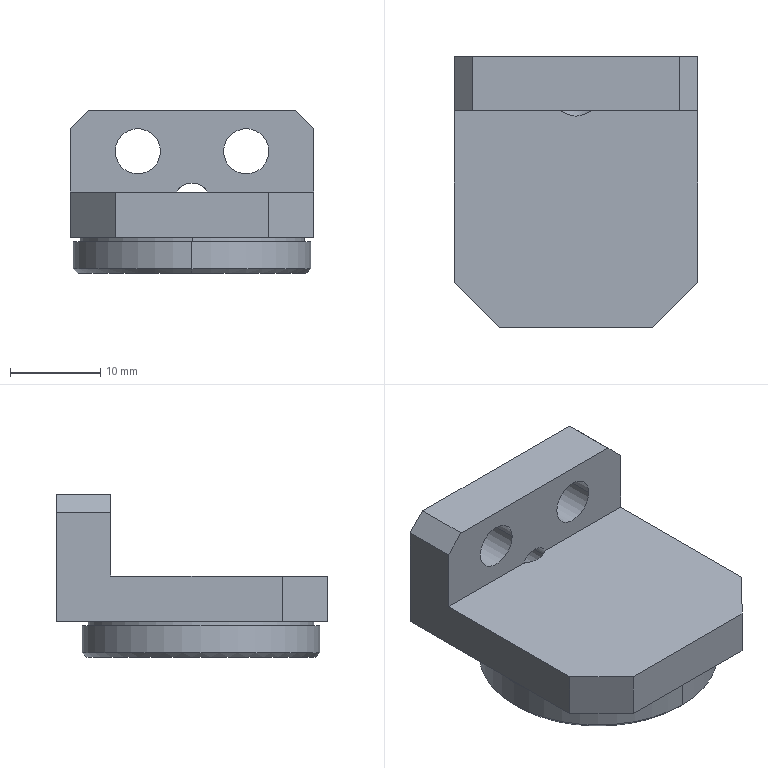NC program | NX | posted with a generic post | part box 27 x 30 x 18 mm
Whole program:
N10 G17 G21 G94 G90
(FLOOR_WALL_COPY , TOOL : D10JING)
N12 T11 M6
N14 G54
N16 G17 G0 G90 X23. Y-13.497 B0. C0. S9500 M3
N18 G43 Z30. H11
N20 Z9.5
N22 G94 G1 Z6.5 F1250.
N24 X20.
N26 X-20.
N28 Y-11.587
N30 Y-8.898
N32 X20.
N34 Y-4.298
N36 X-20.
N38 Y0.301
N40 X20.
N42 Y4.901
N44 X-20.
N46 Y9.5
N48 X20.
N50 X23.
N52 Z9.5
N54 G0 Z30.
N56 Y-13.497
N58 Z9.
N60 G1 Z6.
N62 X20.
N64 X-20.
N66 Y-11.587
N68 Y-8.898
N70 X20.
N72 Y-4.298
N74 X-20.
N76 Y0.301
N78 X20.
N80 Y4.901
N82 X-20.
N84 Y9.5
N86 X20.
N88 X23.
N90 Z9.
N92 G0 Z30.
N94 Y-13.497
N96 Z8.5
N98 G1 Z5.5
N100 X20.
N102 X-20.
N104 Y-11.587
N106 Y-8.898
N108 X20.
N110 Y-4.298
N112 X-20.
N114 Y0.301
N116 X20.
N118 Y4.901
N120 X-20.
N122 Y9.5
N124 X20.
N126 X23.
N128 Z8.5
N130 G0 Z30.
N132 Y-13.497
N134 Z8.
N136 G1 Z5.
N138 X20.
N140 X-20.
N142 Y-11.587
N144 Y-8.898
N146 X20.
N148 Y-4.298
N150 X-20.
N152 Y0.301
N154 X20.
N156 Y4.901
N158 X-20.
N160 Y9.5
N162 X20.
N164 X23.
N166 Z8.
N168 G0 Z30.
N170 Y-13.497
N172 Z7.5
N174 G1 Z4.5
N176 X20.
N178 X-20.
N180 Y-8.898
N182 X20.
N184 Y-4.298
N186 X-20.
N188 Y0.301
N190 X20.
N192 Y4.901
N194 X-20.
N196 Y9.5
N198 X20.
N200 X23.
N202 Z7.5
N204 G0 Z30.
N206 Y-13.497
N208 Z7.
N210 G1 Z4.
N212 X20.
N214 X-20.
N216 Y-8.898
N218 X20.
N220 Y-4.298
N222 X-20.
N224 Y0.301
N226 X20.
N228 Y4.901
N230 X-20.
N232 Y9.5
N234 X20.
N236 X23.
N238 Z7.
N240 G0 Z30.
N242 Y-13.497
N244 Z6.5
N246 G1 Z3.5
N248 X20.
N250 X-20.
N252 Y-8.898
N254 X20.
N256 Y-4.298
N258 X-20.
N260 Y0.301
N262 X20.
N264 Y4.901
N266 X-20.
N268 Y9.5
N270 X20.
N272 X23.
N274 Z6.5
N276 G0 Z30.
N278 Y-13.497
N280 Z6.
N282 G1 Z3.
N284 X20.
N286 X-20.
N288 Y-8.898
N290 X20.
N292 Y-4.298
N294 X-20.
N296 Y0.301
N298 X20.
N300 Y4.901
N302 X-20.
N304 Y9.5
N306 X20.
N308 X23.
N310 Z6.
N312 G0 Z30.
N314 Y-13.497
N316 Z5.5
N318 G1 Z2.5
N320 X20.
N322 X-20.
N324 Y-8.898
N326 X20.
N328 Y-4.298
N330 X-20.
N332 Y0.301
N334 X20.
N336 Y4.901
N338 X-20.
N340 Y9.5
N342 X20.
N344 X23.
N346 Z5.5
N348 G0 Z30.
N350 Y-13.497
N352 Z5.
N354 G1 Z2.
N356 X20.
N358 X-20.
N360 Y-8.898
N362 X20.
N364 Y-4.298
N366 X-20.
N368 Y0.301
N370 X20.
N372 Y4.901
N374 X-20.
N376 Y9.5
N378 X20.
N380 X23.
N382 Z5.
N384 G0 Z30.
N386 Y-13.497
N388 Z4.5
N390 G1 Z1.5
N392 X20.
N394 X-20.
N396 Y-8.898
N398 X20.
N400 Y-4.298
N402 X-20.
N404 Y0.301
N406 X20.
N408 Y4.901
N410 X-20.
N412 Y9.5
N414 X20.
N416 X23.
N418 Z4.5
N420 G0 Z30.
N422 Y-13.497
N424 Z4.
N426 G1 Z1.
N428 X20.
N430 X-20.
N432 Y-8.898
N434 X20.
N436 Y-4.298
N438 X-20.
N440 Y0.301
N442 X20.
N444 Y4.901
N446 X-20.
N448 Y9.5
N450 X20.
N452 X23.
N454 Z4.
N456 G0 Z30.
N458 Y-13.497
N460 Z3.5
N462 G1 Z0.5
N464 X20.
N466 X-20.
N468 Y-8.898
N470 X20.
N472 Y-4.298
N474 X-20.
N476 Y0.301
N478 X20.
N480 Y4.901
N482 X-20.
N484 Y9.5
N486 X20.
N488 X23.
N490 Z3.5
N492 G0 Z30.
N494 Y-13.497
N496 Z3.
N498 G1 Z0.
N500 X20.
N502 X-20.
N504 Y-8.898
N506 X20.
N508 Y-4.298
N510 X-20.
N512 Y0.301
N514 X20.
N516 Y4.901
N518 X-20.
N520 Y9.5
N522 X20.
N524 X23.
N526 Z3.
N528 G0 Z30.
N530 M5
(ZLEVEL_PROFILE_COPY , TOOL : D10)
N532 T10 M6
N534 G54
N536 G17 G0 G90 X16.827 Y9.07 B0. C0. S9500 M3
N538 G43 Z30. H10
N540 Z1.5
N542 G94 G1 X17.37 Y8.078 Z1.441 F1000.
N544 X17.997 Y6.66 Z1.359
N546 X18.501 Y5.193 Z1.278
N548 X18.878 Y3.689 Z1.197
N550 X19.127 Y2.158 Z1.116
N552 X19.245 Y0.611 Z1.034
N554 Y-0.597 Z0.971
N556 X19.11 Y-2.297 Z0.882
N558 X18.817 Y-3.977 Z0.792
N560 X18.368 Y-5.622 Z0.703
N562 X17.767 Y-7.219 Z0.614
N564 X17.02 Y-8.752 Z0.524
N566 X16.134 Y-10.209 Z0.435
N568 X15.115 Y-11.576 Z0.345
N570 X13.973 Y-12.843 Z0.256
N572 X12.718 Y-13.998 Z0.167
N574 X11.361 Y-15.03 Z0.077
N576 X10.796 Y-15.392 Z0.042
N578 X10.229 Y-15.75 Z0.007
N580 X8.895 Y-16.46 Z-0.072
N582 X7.506 Y-17.056 Z-0.151
N584 X6.073 Y-17.536 Z-0.231
N586 X4.604 Y-17.896 Z-0.31
N588 X3.112 Y-18.132 Z-0.389
N590 X1.604 Y-18.245 Z-0.468
N592 X1. Z-0.5
N594 G2 X-17.245 Y0. R18.245 F3000.
N596 X1. Y-18.245 R-18.245
N598 G1 X0.776 Y-18.244 Z-0.504
N600 X0.552 Y-18.24 Z-0.508
N602 X0.329 Y-18.233 Z-0.512
N604 X0.105 Y-18.223 Z-0.516
N606 X-0.118 Y-18.211 Z-0.52
N608 X-0.342 Y-18.196 Z-0.523
N610 X-0.565 Y-18.178 Z-0.527
N612 X-0.787 Y-18.157 Z-0.531
N614 X-1.01 Y-18.134 Z-0.535
N616 X-1.232 Y-18.108 Z-0.539
N618 X-1.454 Y-18.079 Z-0.543
N620 X-1.676 Y-18.048 Z-0.547
N622 X-1.897 Y-18.014 Z-0.551
N624 X-2.118 Y-17.977 Z-0.555
N626 X-2.338 Y-17.937 Z-0.559
N628 X-2.558 Y-17.895 Z-0.563
N630 X-2.777 Y-17.85 Z-0.566
N632 X-2.996 Y-17.802 Z-0.57
N634 X-3.214 Y-17.752 Z-0.574
N636 X-3.431 Y-17.699 Z-0.578
N638 X-3.648 Y-17.643 Z-0.582
N640 X-3.864 Y-17.585 Z-0.586
N642 X-4.079 Y-17.524 Z-0.59
N644 X-4.294 Y-17.46 Z-0.594
N646 X-4.507 Y-17.394 Z-0.598
N648 X-4.72 Y-17.325 Z-0.602
N650 X-4.932 Y-17.254 Z-0.605
N652 X-5.144 Y-17.18 Z-0.609
N654 X-5.354 Y-17.103 Z-0.613
N656 X-5.563 Y-17.024 Z-0.617
N658 X-5.772 Y-16.942 Z-0.621
N660 X-5.979 Y-16.858 Z-0.625
N662 X-6.185 Y-16.771 Z-0.629
N664 X-6.39 Y-16.681 Z-0.633
N666 X-6.594 Y-16.589 Z-0.637
N668 X-6.797 Y-16.495 Z-0.641
N670 X-6.999 Y-16.398 Z-0.645
N672 X-7.199 Y-16.299 Z-0.648
N674 X-7.399 Y-16.197 Z-0.652
N676 X-7.597 Y-16.093 Z-0.656
N678 X-7.793 Y-15.986 Z-0.66
N680 X-7.989 Y-15.877 Z-0.664
N682 X-8.183 Y-15.766 Z-0.668
N684 X-8.376 Y-15.652 Z-0.672
N686 X-8.567 Y-15.536 Z-0.676
N688 X-8.757 Y-15.417 Z-0.68
N690 X-8.945 Y-15.296 Z-0.684
N692 X-9.132 Y-15.173 Z-0.688
N694 X-9.317 Y-15.048 Z-0.691
N696 X-9.501 Y-14.92 Z-0.695
N698 X-9.683 Y-14.79 Z-0.699
N700 X-9.864 Y-14.658 Z-0.703
N702 X-10.043 Y-14.524 Z-0.707
N704 X-10.22 Y-14.387 Z-0.711
N706 X-10.396 Y-14.248 Z-0.715
N708 X-10.57 Y-14.108 Z-0.719
N710 X-10.742 Y-13.965 Z-0.723
N712 X-10.912 Y-13.819 Z-0.727
N714 X-11.081 Y-13.672 Z-0.73
N716 X-11.248 Y-13.523 Z-0.734
N718 X-11.413 Y-13.372 Z-0.738
N720 X-11.576 Y-13.219 Z-0.742
N722 X-11.737 Y-13.063 Z-0.746
N724 X-11.896 Y-12.906 Z-0.75
N726 X-12.053 Y-12.747 Z-0.754
N728 X-12.209 Y-12.586 Z-0.758
N730 X-12.362 Y-12.423 Z-0.762
N732 X-12.514 Y-12.258 Z-0.766
N734 X-12.663 Y-12.092 Z-0.77
N736 X-12.81 Y-11.923 Z-0.773
N738 X-12.955 Y-11.753 Z-0.777
N740 X-13.099 Y-11.581 Z-0.781
N742 X-13.239 Y-11.407 Z-0.785
N744 X-13.378 Y-11.231 Z-0.789
N746 X-13.515 Y-11.054 Z-0.793
N748 X-13.649 Y-10.875 Z-0.797
N750 X-13.782 Y-10.695 Z-0.801
N752 X-13.912 Y-10.513 Z-0.805
N754 X-14.04 Y-10.329 Z-0.809
N756 X-14.165 Y-10.144 Z-0.813
N758 X-14.289 Y-9.957 Z-0.816
N760 X-14.41 Y-9.769 Z-0.82
N762 X-14.528 Y-9.579 Z-0.824
N764 X-14.644 Y-9.388 Z-0.828
N766 X-14.758 Y-9.195 Z-0.832
N768 X-14.87 Y-9.001 Z-0.836
N770 X-14.979 Y-8.806 Z-0.84
N772 X-15.086 Y-8.609 Z-0.844
N774 X-15.19 Y-8.411 Z-0.848
N776 X-15.292 Y-8.212 Z-0.852
N778 X-15.392 Y-8.012 Z-0.855
N780 X-15.489 Y-7.81 Z-0.859
N782 X-15.583 Y-7.607 Z-0.863
N784 X-15.676 Y-7.403 Z-0.867
N786 X-15.765 Y-7.198 Z-0.871
N788 X-15.852 Y-6.992 Z-0.875
N790 X-15.937 Y-6.785 Z-0.879
N792 X-16.019 Y-6.576 Z-0.883
N794 X-16.098 Y-6.367 Z-0.887
N796 X-16.175 Y-6.157 Z-0.891
N798 X-16.249 Y-5.946 Z-0.895
N800 X-16.321 Y-5.734 Z-0.898
N802 X-16.39 Y-5.521 Z-0.902
N804 X-16.456 Y-5.307 Z-0.906
N806 X-16.52 Y-5.093 Z-0.91
N808 X-16.581 Y-4.878 Z-0.914
N810 X-16.639 Y-4.662 Z-0.918
N812 X-16.695 Y-4.445 Z-0.922
N814 X-16.748 Y-4.227 Z-0.926
N816 X-16.799 Y-4.009 Z-0.93
N818 X-16.847 Y-3.791 Z-0.934
N820 X-16.892 Y-3.572 Z-0.938
N822 X-16.934 Y-3.352 Z-0.941
N824 X-16.974 Y-3.132 Z-0.945
N826 X-17.011 Y-2.911 Z-0.949
N828 X-17.046 Y-2.69 Z-0.953
N830 X-17.077 Y-2.468 Z-0.957
N832 X-17.106 Y-2.246 Z-0.961
N834 X-17.132 Y-2.024 Z-0.965
N836 X-17.156 Y-1.802 Z-0.969
N838 X-17.177 Y-1.579 Z-0.973
N840 X-17.195 Y-1.356 Z-0.977
N842 X-17.21 Y-1.132 Z-0.98
N844 X-17.222 Y-0.909 Z-0.984
N846 X-17.232 Y-0.685 Z-0.988
N848 X-17.239 Y-0.462 Z-0.992
N850 X-17.243 Y-0.238 Z-0.996
N852 X-17.245 Y-0.014 Z-1.
N854 Y0.007
N856 G2 X1. Y-18.245 R-18.245
N858 G1 X0.776 Y-18.244 Z-1.004
N860 X0.552 Y-18.24 Z-1.008
N862 X0.329 Y-18.233 Z-1.012
N864 X0.105 Y-18.223 Z-1.016
N866 X-0.118 Y-18.211 Z-1.02
N868 X-0.342 Y-18.196 Z-1.023
N870 X-0.565 Y-18.178 Z-1.027
N872 X-0.787 Y-18.157 Z-1.031
N874 X-1.01 Y-18.134 Z-1.035
N876 X-1.232 Y-18.108 Z-1.039
N878 X-1.454 Y-18.079 Z-1.043
N880 X-1.676 Y-18.048 Z-1.047
N882 X-1.897 Y-18.014 Z-1.051
N884 X-2.118 Y-17.977 Z-1.055
N886 X-2.338 Y-17.937 Z-1.059
N888 X-2.558 Y-17.895 Z-1.063
N890 X-2.777 Y-17.85 Z-1.066
N892 X-2.996 Y-17.802 Z-1.07
N894 X-3.214 Y-17.752 Z-1.074
N896 X-3.431 Y-17.699 Z-1.078
N898 X-3.648 Y-17.643 Z-1.082
N900 X-3.864 Y-17.585 Z-1.086
N902 X-4.079 Y-17.524 Z-1.09
N904 X-4.294 Y-17.46 Z-1.094
N906 X-4.507 Y-17.394 Z-1.098
N908 X-4.72 Y-17.325 Z-1.102
N910 X-4.932 Y-17.254 Z-1.105
N912 X-5.144 Y-17.18 Z-1.109
N914 X-5.354 Y-17.103 Z-1.113
N916 X-5.563 Y-17.024 Z-1.117
N918 X-5.772 Y-16.942 Z-1.121
N920 X-5.979 Y-16.858 Z-1.125
N922 X-6.185 Y-16.771 Z-1.129
N924 X-6.39 Y-16.681 Z-1.133
N926 X-6.594 Y-16.589 Z-1.137
N928 X-6.797 Y-16.495 Z-1.141
N930 X-6.999 Y-16.398 Z-1.145
N932 X-7.199 Y-16.299 Z-1.148
N934 X-7.399 Y-16.197 Z-1.152
N936 X-7.597 Y-16.093 Z-1.156
N938 X-7.793 Y-15.986 Z-1.16
N940 X-7.989 Y-15.877 Z-1.164
N942 X-8.183 Y-15.766 Z-1.168
N944 X-8.376 Y-15.652 Z-1.172
N946 X-8.567 Y-15.536 Z-1.176
N948 X-8.757 Y-15.417 Z-1.18
N950 X-8.945 Y-15.296 Z-1.184
N952 X-9.132 Y-15.173 Z-1.188
N954 X-9.317 Y-15.048 Z-1.191
N956 X-9.501 Y-14.92 Z-1.195
N958 X-9.683 Y-14.79 Z-1.199
N960 X-9.864 Y-14.658 Z-1.203
N962 X-10.043 Y-14.524 Z-1.207
N964 X-10.22 Y-14.387 Z-1.211
N966 X-10.396 Y-14.248 Z-1.215
N968 X-10.57 Y-14.108 Z-1.219
N970 X-10.742 Y-13.965 Z-1.223
N972 X-10.912 Y-13.819 Z-1.227
N974 X-11.081 Y-13.672 Z-1.23
N976 X-11.248 Y-13.523 Z-1.234
N978 X-11.413 Y-13.372 Z-1.238
N980 X-11.576 Y-13.219 Z-1.242
N982 X-11.737 Y-13.063 Z-1.246
N984 X-11.896 Y-12.906 Z-1.25
N986 X-12.053 Y-12.747 Z-1.254
N988 X-12.209 Y-12.586 Z-1.258
N990 X-12.362 Y-12.423 Z-1.262
N992 X-12.514 Y-12.258 Z-1.266
N994 X-12.663 Y-12.092 Z-1.27
N996 X-12.81 Y-11.923 Z-1.273
N998 X-12.955 Y-11.753 Z-1.277
N1000 X-13.099 Y-11.581 Z-1.281
N1002 X-13.239 Y-11.407 Z-1.285
N1004 X-13.378 Y-11.231 Z-1.289
N1006 X-13.515 Y-11.054 Z-1.293
N1008 X-13.649 Y-10.875 Z-1.297
N1010 X-13.782 Y-10.695 Z-1.301
N1012 X-13.912 Y-10.513 Z-1.305
N1014 X-14.04 Y-10.329 Z-1.309
N1016 X-14.165 Y-10.144 Z-1.313
N1018 X-14.289 Y-9.957 Z-1.316
N1020 X-14.41 Y-9.769 Z-1.32
N1022 X-14.528 Y-9.579 Z-1.324
N1024 X-14.644 Y-9.388 Z-1.328
N1026 X-14.758 Y-9.195 Z-1.332
N1028 X-14.87 Y-9.001 Z-1.336
N1030 X-14.979 Y-8.806 Z-1.34
N1032 X-15.086 Y-8.609 Z-1.344
N1034 X-15.19 Y-8.411 Z-1.348
N1036 X-15.292 Y-8.212 Z-1.352
N1038 X-15.392 Y-8.012 Z-1.355
N1040 X-15.489 Y-7.81 Z-1.359
N1042 X-15.583 Y-7.607 Z-1.363
N1044 X-15.676 Y-7.403 Z-1.367
N1046 X-15.765 Y-7.198 Z-1.371
N1048 X-15.852 Y-6.992 Z-1.375
N1050 X-15.937 Y-6.785 Z-1.379
N1052 X-16.019 Y-6.576 Z-1.383
N1054 X-16.098 Y-6.367 Z-1.387
N1056 X-16.175 Y-6.157 Z-1.391
N1058 X-16.249 Y-5.946 Z-1.395
N1060 X-16.321 Y-5.734 Z-1.398
N1062 X-16.39 Y-5.521 Z-1.402
N1064 X-16.456 Y-5.307 Z-1.406
N1066 X-16.52 Y-5.093 Z-1.41
N1068 X-16.581 Y-4.878 Z-1.414
N1070 X-16.639 Y-4.662 Z-1.418
N1072 X-16.695 Y-4.445 Z-1.422
N1074 X-16.748 Y-4.227 Z-1.426
N1076 X-16.799 Y-4.009 Z-1.43
N1078 X-16.847 Y-3.791 Z-1.434
N1080 X-16.892 Y-3.572 Z-1.438
N1082 X-16.934 Y-3.352 Z-1.441
N1084 X-16.974 Y-3.132 Z-1.445
N1086 X-17.011 Y-2.911 Z-1.449
N1088 X-17.046 Y-2.69 Z-1.453
N1090 X-17.077 Y-2.468 Z-1.457
N1092 X-17.106 Y-2.246 Z-1.461
N1094 X-17.132 Y-2.024 Z-1.465
N1096 X-17.156 Y-1.802 Z-1.469
N1098 X-17.177 Y-1.579 Z-1.473
N1100 X-17.195 Y-1.356 Z-1.477
N1102 X-17.21 Y-1.132 Z-1.48
N1104 X-17.222 Y-0.909 Z-1.484
N1106 X-17.232 Y-0.685 Z-1.488
N1108 X-17.239 Y-0.462 Z-1.492
N1110 X-17.243 Y-0.238 Z-1.496
N1112 X-17.245 Y-0.014 Z-1.5
N1114 Y0.007
N1116 G2 X1. Y-18.245 R-18.245
N1118 G1 X0.776 Y-18.244 Z-1.504
N1120 X0.552 Y-18.24 Z-1.508
N1122 X0.329 Y-18.233 Z-1.512
N1124 X0.105 Y-18.223 Z-1.516
N1126 X-0.118 Y-18.211 Z-1.52
N1128 X-0.342 Y-18.196 Z-1.523
N1130 X-0.565 Y-18.178 Z-1.527
N1132 X-0.787 Y-18.157 Z-1.531
N1134 X-1.01 Y-18.134 Z-1.535
N1136 X-1.232 Y-18.108 Z-1.539
N1138 X-1.454 Y-18.079 Z-1.543
N1140 X-1.676 Y-18.048 Z-1.547
N1142 X-1.897 Y-18.014 Z-1.551
N1144 X-2.118 Y-17.977 Z-1.555
N1146 X-2.338 Y-17.937 Z-1.559
N1148 X-2.558 Y-17.895 Z-1.563
N1150 X-2.777 Y-17.85 Z-1.566
N1152 X-2.996 Y-17.802 Z-1.57
N1154 X-3.214 Y-17.752 Z-1.574
N1156 X-3.431 Y-17.699 Z-1.578
N1158 X-3.648 Y-17.643 Z-1.582
N1160 X-3.864 Y-17.585 Z-1.586
N1162 X-4.079 Y-17.524 Z-1.59
N1164 X-4.294 Y-17.46 Z-1.594
N1166 X-4.507 Y-17.394 Z-1.598
N1168 X-4.72 Y-17.325 Z-1.602
N1170 X-4.932 Y-17.254 Z-1.605
N1172 X-5.144 Y-17.18 Z-1.609
N1174 X-5.354 Y-17.103 Z-1.613
N1176 X-5.563 Y-17.024 Z-1.617
N1178 X-5.772 Y-16.942 Z-1.621
N1180 X-5.979 Y-16.858 Z-1.625
N1182 X-6.185 Y-16.771 Z-1.629
N1184 X-6.39 Y-16.681 Z-1.633
N1186 X-6.594 Y-16.589 Z-1.637
N1188 X-6.797 Y-16.495 Z-1.641
N1190 X-6.999 Y-16.398 Z-1.645
N1192 X-7.199 Y-16.299 Z-1.648
N1194 X-7.399 Y-16.197 Z-1.652
N1196 X-7.597 Y-16.093 Z-1.656
N1198 X-7.793 Y-15.986 Z-1.66
N1200 X-7.989 Y-15.877 Z-1.664
N1202 X-8.183 Y-15.766 Z-1.668
N1204 X-8.376 Y-15.652 Z-1.672
N1206 X-8.567 Y-15.536 Z-1.676
N1208 X-8.757 Y-15.417 Z-1.68
N1210 X-8.945 Y-15.296 Z-1.684
N1212 X-9.132 Y-15.173 Z-1.688
N1214 X-9.317 Y-15.048 Z-1.691
N1216 X-9.501 Y-14.92 Z-1.695
N1218 X-9.683 Y-14.79 Z-1.699
N1220 X-9.864 Y-14.658 Z-1.703
N1222 X-10.043 Y-14.524 Z-1.707
N1224 X-10.22 Y-14.387 Z-1.711
N1226 X-10.396 Y-14.248 Z-1.715
N1228 X-10.57 Y-14.108 Z-1.719
N1230 X-10.742 Y-13.965 Z-1.723
N1232 X-10.912 Y-13.819 Z-1.727
N1234 X-11.081 Y-13.672 Z-1.73
N1236 X-11.248 Y-13.523 Z-1.734
N1238 X-11.413 Y-13.372 Z-1.738
N1240 X-11.576 Y-13.219 Z-1.742
N1242 X-11.737 Y-13.063 Z-1.746
N1244 X-11.896 Y-12.906 Z-1.75
N1246 X-12.053 Y-12.747 Z-1.754
N1248 X-12.209 Y-12.586 Z-1.758
N1250 X-12.362 Y-12.423 Z-1.762
N1252 X-12.514 Y-12.258 Z-1.766
N1254 X-12.663 Y-12.092 Z-1.77
N1256 X-12.81 Y-11.923 Z-1.773
N1258 X-12.955 Y-11.753 Z-1.777
N1260 X-13.099 Y-11.581 Z-1.781
N1262 X-13.239 Y-11.407 Z-1.785
N1264 X-13.378 Y-11.231 Z-1.789
N1266 X-13.515 Y-11.054 Z-1.793
N1268 X-13.649 Y-10.875 Z-1.797
N1270 X-13.782 Y-10.695 Z-1.801
N1272 X-13.912 Y-10.513 Z-1.805
N1274 X-14.04 Y-10.329 Z-1.809
N1276 X-14.165 Y-10.144 Z-1.813
N1278 X-14.289 Y-9.957 Z-1.816
N1280 X-14.41 Y-9.769 Z-1.82
N1282 X-14.528 Y-9.579 Z-1.824
N1284 X-14.644 Y-9.388 Z-1.828
N1286 X-14.758 Y-9.195 Z-1.832
N1288 X-14.87 Y-9.001 Z-1.836
N1290 X-14.979 Y-8.806 Z-1.84
N1292 X-15.086 Y-8.609 Z-1.844
N1294 X-15.19 Y-8.411 Z-1.848
N1296 X-15.292 Y-8.212 Z-1.852
N1298 X-15.392 Y-8.012 Z-1.855
N1300 X-15.489 Y-7.81 Z-1.859
N1302 X-15.583 Y-7.607 Z-1.863
N1304 X-15.676 Y-7.403 Z-1.867
N1306 X-15.765 Y-7.198 Z-1.871
N1308 X-15.852 Y-6.992 Z-1.875
N1310 X-15.937 Y-6.785 Z-1.879
N1312 X-16.019 Y-6.576 Z-1.883
N1314 X-16.098 Y-6.367 Z-1.887
N1316 X-16.175 Y-6.157 Z-1.891
N1318 X-16.249 Y-5.946 Z-1.895
N1320 X-16.321 Y-5.734 Z-1.898
N1322 X-16.39 Y-5.521 Z-1.902
N1324 X-16.456 Y-5.307 Z-1.906
N1326 X-16.52 Y-5.093 Z-1.91
N1328 X-16.581 Y-4.878 Z-1.914
N1330 X-16.639 Y-4.662 Z-1.918
N1332 X-16.695 Y-4.445 Z-1.922
N1334 X-16.748 Y-4.227 Z-1.926
N1336 X-16.799 Y-4.009 Z-1.93
N1338 X-16.847 Y-3.791 Z-1.934
N1340 X-16.892 Y-3.572 Z-1.938
N1342 X-16.934 Y-3.352 Z-1.941
N1344 X-16.974 Y-3.132 Z-1.945
N1346 X-17.011 Y-2.911 Z-1.949
N1348 X-17.046 Y-2.69 Z-1.953
N1350 X-17.077 Y-2.468 Z-1.957
N1352 X-17.106 Y-2.246 Z-1.961
N1354 X-17.132 Y-2.024 Z-1.965
N1356 X-17.156 Y-1.802 Z-1.969
N1358 X-17.177 Y-1.579 Z-1.973
N1360 X-17.195 Y-1.356 Z-1.977
N1362 X-17.21 Y-1.132 Z-1.98
N1364 X-17.222 Y-0.909 Z-1.984
N1366 X-17.232 Y-0.685 Z-1.988
N1368 X-17.239 Y-0.462 Z-1.992
N1370 X-17.243 Y-0.238 Z-1.996
N1372 X-17.245 Y-0.014 Z-2.
N1374 Y0.007
N1376 G2 X1. Y-18.245 R-18.245
N1378 G1 X0.776 Y-18.244 Z-2.004
N1380 X0.552 Y-18.24 Z-2.008
N1382 X0.329 Y-18.233 Z-2.012
N1384 X0.105 Y-18.223 Z-2.016
N1386 X-0.118 Y-18.211 Z-2.02
N1388 X-0.342 Y-18.196 Z-2.023
N1390 X-0.565 Y-18.178 Z-2.027
N1392 X-0.787 Y-18.157 Z-2.031
N1394 X-1.01 Y-18.134 Z-2.035
N1396 X-1.232 Y-18.108 Z-2.039
N1398 X-1.454 Y-18.079 Z-2.043
N1400 X-1.676 Y-18.048 Z-2.047
N1402 X-1.897 Y-18.014 Z-2.051
N1404 X-2.118 Y-17.977 Z-2.055
N1406 X-2.338 Y-17.937 Z-2.059
N1408 X-2.558 Y-17.895 Z-2.063
N1410 X-2.777 Y-17.85 Z-2.066
N1412 X-2.996 Y-17.802 Z-2.07
N1414 X-3.214 Y-17.752 Z-2.074
N1416 X-3.431 Y-17.699 Z-2.078
N1418 X-3.648 Y-17.643 Z-2.082
N1420 X-3.864 Y-17.585 Z-2.086
N1422 X-4.079 Y-17.524 Z-2.09
N1424 X-4.294 Y-17.46 Z-2.094
N1426 X-4.507 Y-17.394 Z-2.098
N1428 X-4.72 Y-17.325 Z-2.102
N1430 X-4.932 Y-17.254 Z-2.105
N1432 X-5.144 Y-17.18 Z-2.109
N1434 X-5.354 Y-17.103 Z-2.113
N1436 X-5.563 Y-17.024 Z-2.117
N1438 X-5.772 Y-16.942 Z-2.121
N1440 X-5.979 Y-16.858 Z-2.125
N1442 X-6.185 Y-16.771 Z-2.129
N1444 X-6.39 Y-16.681 Z-2.133
N1446 X-6.594 Y-16.589 Z-2.137
N1448 X-6.797 Y-16.495 Z-2.141
N1450 X-6.999 Y-16.398 Z-2.145
N1452 X-7.199 Y-16.299 Z-2.148
N1454 X-7.399 Y-16.197 Z-2.152
N1456 X-7.597 Y-16.093 Z-2.156
N1458 X-7.793 Y-15.986 Z-2.16
N1460 X-7.989 Y-15.877 Z-2.164
N1462 X-8.183 Y-15.766 Z-2.168
N1464 X-8.376 Y-15.652 Z-2.172
N1466 X-8.567 Y-15.536 Z-2.176
N1468 X-8.757 Y-15.417 Z-2.18
N1470 X-8.945 Y-15.296 Z-2.184
N1472 X-9.132 Y-15.173 Z-2.188
N1474 X-9.317 Y-15.048 Z-2.191
N1476 X-9.501 Y-14.92 Z-2.195
N1478 X-9.683 Y-14.79 Z-2.199
N1480 X-9.864 Y-14.658 Z-2.203
N1482 X-10.043 Y-14.524 Z-2.207
N1484 X-10.22 Y-14.387 Z-2.211
N1486 X-10.396 Y-14.248 Z-2.215
N1488 X-10.57 Y-14.108 Z-2.219
N1490 X-10.742 Y-13.965 Z-2.223
N1492 X-10.912 Y-13.819 Z-2.227
N1494 X-11.081 Y-13.672 Z-2.23
N1496 X-11.248 Y-13.523 Z-2.234
N1498 X-11.413 Y-13.372 Z-2.238
N1500 X-11.576 Y-13.219 Z-2.242
N1502 X-11.737 Y-13.063 Z-2.246
N1504 X-11.896 Y-12.906 Z-2.25
N1506 X-12.053 Y-12.747 Z-2.254
N1508 X-12.209 Y-12.586 Z-2.258
N1510 X-12.362 Y-12.423 Z-2.262
N1512 X-12.514 Y-12.258 Z-2.266
N1514 X-12.663 Y-12.092 Z-2.27
N1516 X-12.81 Y-11.923 Z-2.273
N1518 X-12.955 Y-11.753 Z-2.277
N1520 X-13.099 Y-11.581 Z-2.281
N1522 X-13.239 Y-11.407 Z-2.285
N1524 X-13.378 Y-11.231 Z-2.289
N1526 X-13.515 Y-11.054 Z-2.293
N1528 X-13.649 Y-10.875 Z-2.297
N1530 X-13.782 Y-10.695 Z-2.301
N1532 X-13.912 Y-10.513 Z-2.305
N1534 X-14.04 Y-10.329 Z-2.309
N1536 X-14.165 Y-10.144 Z-2.313
N1538 X-14.289 Y-9.957 Z-2.316
N1540 X-14.41 Y-9.769 Z-2.32
N1542 X-14.528 Y-9.579 Z-2.324
N1544 X-14.644 Y-9.388 Z-2.328
N1546 X-14.758 Y-9.195 Z-2.332
N1548 X-14.87 Y-9.001 Z-2.336
N1550 X-14.979 Y-8.806 Z-2.34
N1552 X-15.086 Y-8.609 Z-2.344
N1554 X-15.19 Y-8.411 Z-2.348
N1556 X-15.292 Y-8.212 Z-2.352
N1558 X-15.392 Y-8.012 Z-2.355
N1560 X-15.489 Y-7.81 Z-2.359
N1562 X-15.583 Y-7.607 Z-2.363
N1564 X-15.676 Y-7.403 Z-2.367
N1566 X-15.765 Y-7.198 Z-2.371
N1568 X-15.852 Y-6.992 Z-2.375
N1570 X-15.937 Y-6.785 Z-2.379
N1572 X-16.019 Y-6.576 Z-2.383
N1574 X-16.098 Y-6.367 Z-2.387
N1576 X-16.175 Y-6.157 Z-2.391
N1578 X-16.249 Y-5.946 Z-2.395
N1580 X-16.321 Y-5.734 Z-2.398
N1582 X-16.39 Y-5.521 Z-2.402
N1584 X-16.456 Y-5.307 Z-2.406
N1586 X-16.52 Y-5.093 Z-2.41
N1588 X-16.581 Y-4.878 Z-2.414
N1590 X-16.639 Y-4.662 Z-2.418
N1592 X-16.695 Y-4.445 Z-2.422
N1594 X-16.748 Y-4.227 Z-2.426
N1596 X-16.799 Y-4.009 Z-2.43
N1598 X-16.847 Y-3.791 Z-2.434
N1600 X-16.892 Y-3.572 Z-2.438
N1602 X-16.934 Y-3.352 Z-2.441
N1604 X-16.974 Y-3.132 Z-2.445
N1606 X-17.011 Y-2.911 Z-2.449
N1608 X-17.046 Y-2.69 Z-2.453
N1610 X-17.077 Y-2.468 Z-2.457
N1612 X-17.106 Y-2.246 Z-2.461
N1614 X-17.132 Y-2.024 Z-2.465
N1616 X-17.156 Y-1.802 Z-2.469
N1618 X-17.177 Y-1.579 Z-2.473
N1620 X-17.195 Y-1.356 Z-2.477
N1622 X-17.21 Y-1.132 Z-2.48
N1624 X-17.222 Y-0.909 Z-2.484
N1626 X-17.232 Y-0.685 Z-2.488
N1628 X-17.239 Y-0.462 Z-2.492
N1630 X-17.243 Y-0.238 Z-2.496
N1632 X-17.245 Y-0.014 Z-2.5
N1634 Y0.007
N1636 G2 X1. Y-18.245 R-18.245
N1638 G1 X0.776 Y-18.244 Z-2.504
N1640 X0.552 Y-18.24 Z-2.508
N1642 X0.329 Y-18.233 Z-2.512
N1644 X0.105 Y-18.223 Z-2.516
N1646 X-0.118 Y-18.211 Z-2.52
N1648 X-0.342 Y-18.196 Z-2.523
N1650 X-0.565 Y-18.178 Z-2.527
N1652 X-0.787 Y-18.157 Z-2.531
N1654 X-1.01 Y-18.134 Z-2.535
N1656 X-1.232 Y-18.108 Z-2.539
N1658 X-1.454 Y-18.079 Z-2.543
N1660 X-1.676 Y-18.048 Z-2.547
N1662 X-1.897 Y-18.014 Z-2.551
N1664 X-2.118 Y-17.977 Z-2.555
N1666 X-2.338 Y-17.937 Z-2.559
N1668 X-2.558 Y-17.895 Z-2.563
N1670 X-2.777 Y-17.85 Z-2.566
N1672 X-2.996 Y-17.802 Z-2.57
N1674 X-3.214 Y-17.752 Z-2.574
N1676 X-3.431 Y-17.699 Z-2.578
N1678 X-3.648 Y-17.643 Z-2.582
N1680 X-3.864 Y-17.585 Z-2.586
N1682 X-4.079 Y-17.524 Z-2.59
N1684 X-4.294 Y-17.46 Z-2.594
N1686 X-4.507 Y-17.394 Z-2.598
N1688 X-4.72 Y-17.325 Z-2.602
N1690 X-4.932 Y-17.254 Z-2.605
N1692 X-5.144 Y-17.18 Z-2.609
N1694 X-5.354 Y-17.103 Z-2.613
N1696 X-5.563 Y-17.024 Z-2.617
N1698 X-5.772 Y-16.942 Z-2.621
N1700 X-5.979 Y-16.858 Z-2.625
N1702 X-6.185 Y-16.771 Z-2.629
N1704 X-6.39 Y-16.681 Z-2.633
N1706 X-6.594 Y-16.589 Z-2.637
N1708 X-6.797 Y-16.495 Z-2.641
N1710 X-6.999 Y-16.398 Z-2.645
N1712 X-7.199 Y-16.299 Z-2.648
N1714 X-7.399 Y-16.197 Z-2.652
N1716 X-7.597 Y-16.093 Z-2.656
N1718 X-7.793 Y-15.986 Z-2.66
N1720 X-7.989 Y-15.877 Z-2.664
N1722 X-8.183 Y-15.766 Z-2.668
N1724 X-8.376 Y-15.652 Z-2.672
N1726 X-8.567 Y-15.536 Z-2.676
N1728 X-8.757 Y-15.417 Z-2.68
N1730 X-8.945 Y-15.296 Z-2.684
N1732 X-9.132 Y-15.173 Z-2.688
N1734 X-9.317 Y-15.048 Z-2.691
N1736 X-9.501 Y-14.92 Z-2.695
N1738 X-9.683 Y-14.79 Z-2.699
N1740 X-9.864 Y-14.658 Z-2.703
N1742 X-10.043 Y-14.524 Z-2.707
N1744 X-10.22 Y-14.387 Z-2.711
N1746 X-10.396 Y-14.248 Z-2.715
N1748 X-10.57 Y-14.108 Z-2.719
N1750 X-10.742 Y-13.965 Z-2.723
N1752 X-10.912 Y-13.819 Z-2.727
N1754 X-11.081 Y-13.672 Z-2.73
N1756 X-11.248 Y-13.523 Z-2.734
N1758 X-11.413 Y-13.372 Z-2.738
N1760 X-11.576 Y-13.219 Z-2.742
N1762 X-11.737 Y-13.063 Z-2.746
N1764 X-11.896 Y-12.906 Z-2.75
N1766 X-12.053 Y-12.747 Z-2.754
N1768 X-12.209 Y-12.586 Z-2.758
N1770 X-12.362 Y-12.423 Z-2.762
N1772 X-12.514 Y-12.258 Z-2.766
N1774 X-12.663 Y-12.092 Z-2.77
N1776 X-12.81 Y-11.923 Z-2.773
N1778 X-12.955 Y-11.753 Z-2.777
N1780 X-13.099 Y-11.581 Z-2.781
N1782 X-13.239 Y-11.407 Z-2.785
N1784 X-13.378 Y-11.231 Z-2.789
N1786 X-13.515 Y-11.054 Z-2.793
N1788 X-13.649 Y-10.875 Z-2.797
N1790 X-13.782 Y-10.695 Z-2.801
N1792 X-13.912 Y-10.513 Z-2.805
N1794 X-14.04 Y-10.329 Z-2.809
N1796 X-14.165 Y-10.144 Z-2.813
N1798 X-14.289 Y-9.957 Z-2.816
N1800 X-14.41 Y-9.769 Z-2.82
N1802 X-14.528 Y-9.579 Z-2.824
N1804 X-14.644 Y-9.388 Z-2.828
N1806 X-14.758 Y-9.195 Z-2.832
N1808 X-14.87 Y-9.001 Z-2.836
N1810 X-14.979 Y-8.806 Z-2.84
N1812 X-15.086 Y-8.609 Z-2.844
N1814 X-15.19 Y-8.411 Z-2.848
N1816 X-15.292 Y-8.212 Z-2.852
N1818 X-15.392 Y-8.012 Z-2.855
N1820 X-15.489 Y-7.81 Z-2.859
N1822 X-15.583 Y-7.607 Z-2.863
N1824 X-15.676 Y-7.403 Z-2.867
N1826 X-15.765 Y-7.198 Z-2.871
N1828 X-15.852 Y-6.992 Z-2.875
N1830 X-15.937 Y-6.785 Z-2.879
N1832 X-16.019 Y-6.576 Z-2.883
N1834 X-16.098 Y-6.367 Z-2.887
N1836 X-16.175 Y-6.157 Z-2.891
N1838 X-16.249 Y-5.946 Z-2.895
N1840 X-16.321 Y-5.734 Z-2.898
N1842 X-16.39 Y-5.521 Z-2.902
N1844 X-16.456 Y-5.307 Z-2.906
N1846 X-16.52 Y-5.093 Z-2.91
N1848 X-16.581 Y-4.878 Z-2.914
N1850 X-16.639 Y-4.662 Z-2.918
N1852 X-16.695 Y-4.445 Z-2.922
N1854 X-16.748 Y-4.227 Z-2.926
N1856 X-16.799 Y-4.009 Z-2.93
N1858 X-16.847 Y-3.791 Z-2.934
N1860 X-16.892 Y-3.572 Z-2.938
N1862 X-16.934 Y-3.352 Z-2.941
N1864 X-16.974 Y-3.132 Z-2.945
N1866 X-17.011 Y-2.911 Z-2.949
N1868 X-17.046 Y-2.69 Z-2.953
N1870 X-17.077 Y-2.468 Z-2.957
N1872 X-17.106 Y-2.246 Z-2.961
N1874 X-17.132 Y-2.024 Z-2.965
N1876 X-17.156 Y-1.802 Z-2.969
N1878 X-17.177 Y-1.579 Z-2.973
N1880 X-17.195 Y-1.356 Z-2.977
N1882 X-17.21 Y-1.132 Z-2.98
N1884 X-17.222 Y-0.909 Z-2.984
N1886 X-17.232 Y-0.685 Z-2.988
N1888 X-17.239 Y-0.462 Z-2.992
N1890 X-17.243 Y-0.238 Z-2.996
N1892 X-17.245 Y-0.014 Z-3.
N1894 Y0.007
N1896 G2 X1. Y-18.245 R-18.245
N1898 G1 X0.776 Y-18.244 Z-3.004
N1900 X0.552 Y-18.24 Z-3.008
N1902 X0.329 Y-18.233 Z-3.012
N1904 X0.105 Y-18.223 Z-3.016
N1906 X-0.118 Y-18.211 Z-3.02
N1908 X-0.342 Y-18.196 Z-3.023
N1910 X-0.565 Y-18.178 Z-3.027
N1912 X-0.787 Y-18.157 Z-3.031
N1914 X-1.01 Y-18.134 Z-3.035
N1916 X-1.232 Y-18.108 Z-3.039
N1918 X-1.454 Y-18.079 Z-3.043
N1920 X-1.676 Y-18.048 Z-3.047
N1922 X-1.897 Y-18.014 Z-3.051
N1924 X-2.118 Y-17.977 Z-3.055
N1926 X-2.338 Y-17.937 Z-3.059
N1928 X-2.558 Y-17.895 Z-3.063
N1930 X-2.777 Y-17.85 Z-3.066
N1932 X-2.996 Y-17.802 Z-3.07
N1934 X-3.214 Y-17.752 Z-3.074
N1936 X-3.431 Y-17.699 Z-3.078
N1938 X-3.648 Y-17.643 Z-3.082
N1940 X-3.864 Y-17.585 Z-3.086
N1942 X-4.079 Y-17.524 Z-3.09
N1944 X-4.294 Y-17.46 Z-3.094
N1946 X-4.507 Y-17.394 Z-3.098
N1948 X-4.72 Y-17.325 Z-3.102
N1950 X-4.932 Y-17.254 Z-3.105
N1952 X-5.144 Y-17.18 Z-3.109
N1954 X-5.354 Y-17.103 Z-3.113
N1956 X-5.563 Y-17.024 Z-3.117
N1958 X-5.772 Y-16.942 Z-3.121
N1960 X-5.979 Y-16.858 Z-3.125
N1962 X-6.185 Y-16.771 Z-3.129
N1964 X-6.39 Y-16.681 Z-3.133
N1966 X-6.594 Y-16.589 Z-3.137
N1968 X-6.797 Y-16.495 Z-3.141
N1970 X-6.999 Y-16.398 Z-3.145
N1972 X-7.199 Y-16.299 Z-3.148
N1974 X-7.399 Y-16.197 Z-3.152
N1976 X-7.597 Y-16.093 Z-3.156
N1978 X-7.793 Y-15.986 Z-3.16
N1980 X-7.989 Y-15.877 Z-3.164
N1982 X-8.183 Y-15.766 Z-3.168
N1984 X-8.376 Y-15.652 Z-3.172
N1986 X-8.567 Y-15.536 Z-3.176
N1988 X-8.757 Y-15.417 Z-3.18
N1990 X-8.945 Y-15.296 Z-3.184
N1992 X-9.132 Y-15.173 Z-3.188
N1994 X-9.317 Y-15.048 Z-3.191
N1996 X-9.501 Y-14.92 Z-3.195
N1998 X-9.683 Y-14.79 Z-3.199
N2000 X-9.864 Y-14.658 Z-3.203
N2002 X-10.043 Y-14.524 Z-3.207
N2004 X-10.22 Y-14.387 Z-3.211
N2006 X-10.396 Y-14.248 Z-3.215
N2008 X-10.57 Y-14.108 Z-3.219
N2010 X-10.742 Y-13.965 Z-3.223
N2012 X-10.912 Y-13.819 Z-3.227
N2014 X-11.081 Y-13.672 Z-3.23
N2016 X-11.248 Y-13.523 Z-3.234
N2018 X-11.413 Y-13.372 Z-3.238
N2020 X-11.576 Y-13.219 Z-3.242
N2022 X-11.737 Y-13.063 Z-3.246
N2024 X-11.896 Y-12.906 Z-3.25
N2026 X-12.053 Y-12.747 Z-3.254
N2028 X-12.209 Y-12.586 Z-3.258
N2030 X-12.362 Y-12.423 Z-3.262
N2032 X-12.514 Y-12.258 Z-3.266
N2034 X-12.663 Y-12.092 Z-3.27
N2036 X-12.81 Y-11.923 Z-3.273
N2038 X-12.955 Y-11.753 Z-3.277
N2040 X-13.099 Y-11.581 Z-3.281
N2042 X-13.239 Y-11.407 Z-3.285
N2044 X-13.378 Y-11.231 Z-3.289
N2046 X-13.515 Y-11.054 Z-3.293
N2048 X-13.649 Y-10.875 Z-3.297
N2050 X-13.782 Y-10.695 Z-3.301
N2052 X-13.912 Y-10.513 Z-3.305
N2054 X-14.04 Y-10.329 Z-3.309
N2056 X-14.165 Y-10.144 Z-3.313
N2058 X-14.289 Y-9.957 Z-3.316
N2060 X-14.41 Y-9.769 Z-3.32
N2062 X-14.528 Y-9.579 Z-3.324
N2064 X-14.644 Y-9.388 Z-3.328
N2066 X-14.758 Y-9.195 Z-3.332
N2068 X-14.87 Y-9.001 Z-3.336
N2070 X-14.979 Y-8.806 Z-3.34
N2072 X-15.086 Y-8.609 Z-3.344
N2074 X-15.19 Y-8.411 Z-3.348
N2076 X-15.292 Y-8.212 Z-3.352
N2078 X-15.392 Y-8.012 Z-3.355
N2080 X-15.489 Y-7.81 Z-3.359
N2082 X-15.583 Y-7.607 Z-3.363
N2084 X-15.676 Y-7.403 Z-3.367
N2086 X-15.765 Y-7.198 Z-3.371
N2088 X-15.852 Y-6.992 Z-3.375
N2090 X-15.937 Y-6.785 Z-3.379
N2092 X-16.019 Y-6.576 Z-3.383
N2094 X-16.098 Y-6.367 Z-3.387
N2096 X-16.175 Y-6.157 Z-3.391
N2098 X-16.249 Y-5.946 Z-3.395
N2100 X-16.321 Y-5.734 Z-3.398
N2102 X-16.39 Y-5.521 Z-3.402
N2104 X-16.456 Y-5.307 Z-3.406
N2106 X-16.52 Y-5.093 Z-3.41
N2108 X-16.581 Y-4.878 Z-3.414
N2110 X-16.639 Y-4.662 Z-3.418
N2112 X-16.695 Y-4.445 Z-3.422
N2114 X-16.748 Y-4.227 Z-3.426
N2116 X-16.799 Y-4.009 Z-3.43
N2118 X-16.847 Y-3.791 Z-3.434
N2120 X-16.892 Y-3.572 Z-3.438
N2122 X-16.934 Y-3.352 Z-3.441
N2124 X-16.974 Y-3.132 Z-3.445
N2126 X-17.011 Y-2.911 Z-3.449
N2128 X-17.046 Y-2.69 Z-3.453
N2130 X-17.077 Y-2.468 Z-3.457
N2132 X-17.106 Y-2.246 Z-3.461
N2134 X-17.132 Y-2.024 Z-3.465
N2136 X-17.156 Y-1.802 Z-3.469
N2138 X-17.177 Y-1.579 Z-3.473
N2140 X-17.195 Y-1.356 Z-3.477
N2142 X-17.21 Y-1.132 Z-3.48
N2144 X-17.222 Y-0.909 Z-3.484
N2146 X-17.232 Y-0.685 Z-3.488
N2148 X-17.239 Y-0.462 Z-3.492
N2150 X-17.243 Y-0.238 Z-3.496
N2152 X-17.245 Y-0.014 Z-3.5
N2154 Y0.007
N2156 G2 X1. Y-18.245 R-18.245
N2158 G1 X0.776 Y-18.244 Z-3.504
N2160 X0.552 Y-18.24 Z-3.508
N2162 X0.329 Y-18.233 Z-3.512
N2164 X0.105 Y-18.223 Z-3.516
N2166 X-0.118 Y-18.211 Z-3.52
N2168 X-0.342 Y-18.196 Z-3.523
N2170 X-0.565 Y-18.178 Z-3.527
N2172 X-0.787 Y-18.157 Z-3.531
N2174 X-1.01 Y-18.134 Z-3.535
N2176 X-1.232 Y-18.108 Z-3.539
N2178 X-1.454 Y-18.079 Z-3.543
N2180 X-1.676 Y-18.048 Z-3.547
N2182 X-1.897 Y-18.014 Z-3.551
N2184 X-2.118 Y-17.977 Z-3.555
N2186 X-2.338 Y-17.937 Z-3.559
N2188 X-2.558 Y-17.895 Z-3.563
N2190 X-2.777 Y-17.85 Z-3.566
N2192 X-2.996 Y-17.802 Z-3.57
N2194 X-3.214 Y-17.752 Z-3.574
N2196 X-3.431 Y-17.699 Z-3.578
N2198 X-3.648 Y-17.643 Z-3.582
N2200 X-3.864 Y-17.585 Z-3.586
N2202 X-4.079 Y-17.524 Z-3.59
N2204 X-4.294 Y-17.46 Z-3.594
N2206 X-4.507 Y-17.394 Z-3.598
N2208 X-4.72 Y-17.325 Z-3.602
N2210 X-4.932 Y-17.254 Z-3.605
N2212 X-5.144 Y-17.18 Z-3.609
N2214 X-5.354 Y-17.103 Z-3.613
N2216 X-5.563 Y-17.024 Z-3.617
N2218 X-5.772 Y-16.942 Z-3.621
N2220 X-5.979 Y-16.858 Z-3.625
N2222 X-6.185 Y-16.771 Z-3.629
N2224 X-6.39 Y-16.681 Z-3.633
N2226 X-6.594 Y-16.589 Z-3.637
N2228 X-6.797 Y-16.495 Z-3.641
N2230 X-6.999 Y-16.398 Z-3.645
N2232 X-7.199 Y-16.299 Z-3.648
N2234 X-7.399 Y-16.197 Z-3.652
N2236 X-7.597 Y-16.093 Z-3.656
N2238 X-7.793 Y-15.986 Z-3.66
N2240 X-7.989 Y-15.877 Z-3.664
N2242 X-8.183 Y-15.766 Z-3.668
N2244 X-8.376 Y-15.652 Z-3.672
N2246 X-8.567 Y-15.536 Z-3.676
N2248 X-8.757 Y-15.417 Z-3.68
N2250 X-8.945 Y-15.296 Z-3.684
N2252 X-9.132 Y-15.173 Z-3.688
N2254 X-9.317 Y-15.048 Z-3.691
N2256 X-9.501 Y-14.92 Z-3.695
N2258 X-9.683 Y-14.79 Z-3.699
N2260 X-9.864 Y-14.658 Z-3.703
N2262 X-10.043 Y-14.524 Z-3.707
N2264 X-10.22 Y-14.387 Z-3.711
N2266 X-10.396 Y-14.248 Z-3.715
N2268 X-10.57 Y-14.108 Z-3.719
N2270 X-10.742 Y-13.965 Z-3.723
N2272 X-10.912 Y-13.819 Z-3.727
N2274 X-11.081 Y-13.672 Z-3.73
N2276 X-11.248 Y-13.523 Z-3.734
N2278 X-11.413 Y-13.372 Z-3.738
N2280 X-11.576 Y-13.219 Z-3.742
N2282 X-11.737 Y-13.063 Z-3.746
N2284 X-11.896 Y-12.906 Z-3.75
N2286 X-12.053 Y-12.747 Z-3.754
N2288 X-12.209 Y-12.586 Z-3.758
N2290 X-12.362 Y-12.423 Z-3.762
N2292 X-12.514 Y-12.258 Z-3.766
N2294 X-12.663 Y-12.092 Z-3.77
N2296 X-12.81 Y-11.923 Z-3.773
N2298 X-12.955 Y-11.753 Z-3.777
N2300 X-13.099 Y-11.581 Z-3.781
N2302 X-13.239 Y-11.407 Z-3.785
N2304 X-13.378 Y-11.231 Z-3.789
N2306 X-13.515 Y-11.054 Z-3.793
N2308 X-13.649 Y-10.875 Z-3.797
N2310 X-13.782 Y-10.695 Z-3.801
N2312 X-13.912 Y-10.513 Z-3.805
N2314 X-14.04 Y-10.329 Z-3.809
N2316 X-14.165 Y-10.144 Z-3.813
N2318 X-14.289 Y-9.957 Z-3.816
N2320 X-14.41 Y-9.769 Z-3.82
N2322 X-14.528 Y-9.579 Z-3.824
N2324 X-14.644 Y-9.388 Z-3.828
N2326 X-14.758 Y-9.195 Z-3.832
N2328 X-14.87 Y-9.001 Z-3.836
N2330 X-14.979 Y-8.806 Z-3.84
N2332 X-15.086 Y-8.609 Z-3.844
N2334 X-15.19 Y-8.411 Z-3.848
N2336 X-15.292 Y-8.212 Z-3.852
N2338 X-15.392 Y-8.012 Z-3.855
N2340 X-15.489 Y-7.81 Z-3.859
N2342 X-15.583 Y-7.607 Z-3.863
N2344 X-15.676 Y-7.403 Z-3.867
N2346 X-15.765 Y-7.198 Z-3.871
N2348 X-15.852 Y-6.992 Z-3.875
N2350 X-15.937 Y-6.785 Z-3.879
N2352 X-16.019 Y-6.576 Z-3.883
N2354 X-16.098 Y-6.367 Z-3.887
N2356 X-16.175 Y-6.157 Z-3.891
N2358 X-16.249 Y-5.946 Z-3.895
N2360 X-16.321 Y-5.734 Z-3.898
N2362 X-16.39 Y-5.521 Z-3.902
N2364 X-16.456 Y-5.307 Z-3.906
N2366 X-16.52 Y-5.093 Z-3.91
N2368 X-16.581 Y-4.878 Z-3.914
N2370 X-16.639 Y-4.662 Z-3.918
N2372 X-16.695 Y-4.445 Z-3.922
N2374 X-16.748 Y-4.227 Z-3.926
N2376 X-16.799 Y-4.009 Z-3.93
N2378 X-16.847 Y-3.791 Z-3.934
N2380 X-16.892 Y-3.572 Z-3.938
N2382 X-16.934 Y-3.352 Z-3.941
N2384 X-16.974 Y-3.132 Z-3.945
N2386 X-17.011 Y-2.911 Z-3.949
N2388 X-17.046 Y-2.69 Z-3.953
N2390 X-17.077 Y-2.468 Z-3.957
N2392 X-17.106 Y-2.246 Z-3.961
N2394 X-17.132 Y-2.024 Z-3.965
N2396 X-17.156 Y-1.802 Z-3.969
N2398 X-17.177 Y-1.579 Z-3.973
N2400 X-17.195 Y-1.356 Z-3.977
N2402 X-17.21 Y-1.132 Z-3.98
N2404 X-17.222 Y-0.909 Z-3.984
N2406 X-17.232 Y-0.685 Z-3.988
N2408 X-17.239 Y-0.462 Z-3.992
N2410 X-17.243 Y-0.238 Z-3.996
N2412 X-17.245 Y-0.014 Z-4.
N2414 Y0.007
N2416 G2 X1.007 Y18.245 R18.245
N2418 X-17.245 Y-0.014 R-18.245
N2420 G1 Z-2.5
N2422 G0 Z30.
N2424 M5
(ZLEVEL_PROFILE_COPY_1_COPY , TOOL : D10JING)
N2426 T11 M6
N2428 G54
N2430 G17 G0 G90 X2.691 Y-20.074 B0. C0. S9500 M3
N2432 G43 Z30. H11
N2434 Z-2.5
N2436 G94 G1 Z-4. F1000.
N2438 X1.866 Y-18.645
N2440 G3 X1. Y-18.145 R1.
N2442 G2 X-17.145 Y0. R18.145 F1200.
N2444 X1. Y-18.145 R-18.145
N2446 G3 X0.134 Y-18.645 R1.
N2448 G1 X-0.691 Y-20.074
N2450 Z-2.5
N2452 G0 Z30.
N2454 M5
(PLANAR_MILL_COPY_COPY_1 , TOOL : D6A45)
N2456 T07 M6
N2458 G54
N2460 G17 G0 G90 X15.793 Y1.24 B0. C0. S9500 M3
N2462 G43 Z30. H7
N2464 Z0.5
N2466 G94 G1 Z-1. F1250.
N2468 X15.145 Y0.866
N2470 G3 X14.645 Y0. R1.
N2472 G2 X1. Y-13.645 R13.645
N2474 X14.645 Y0. R-13.645
N2476 G3 X15.145 Y-0.866 R1.
N2478 G1 X15.793 Y-1.24
N2480 Z0.5
N2482 G0 Z30.
N2484 M5
(PLANAR_MILL , TOOL : T8H0.5)
N2486 T08 M6
N2488 G54
N2490 G17 G0 G90 X21.27 Y5.859 B0. C0. S5000 M3
N2492 G43 Z30. H8
N2494 Z-1.
N2496 G94 G1 Z-4. F1000.
N2498 G3 X18.1 Y0. R7.
N2500 G2 X1. Y-17.1 R17.1
N2502 X18.1 Y0. R-17.1
N2504 G3 X21.27 Y-5.859 R7.
N2506 G1 X21.262 Y5.887
N2508 G3 X18.05 Y0. R7.
N2510 G2 X1. Y-17.05 R17.05
N2512 X18.05 Y0. R-17.05
N2514 G3 X21.218 Y-5.858 R7.
N2516 G1 X21.21 Y5.886
N2518 G3 X18. Y0. R7.
N2520 G2 X1. Y-17. R17.
N2522 X18. Y0. R-17.
N2524 G3 X21.167 Y-5.857 R7.
N2526 G1 X21.159 Y5.884
N2528 G3 X17.95 Y0. R7.
N2530 G2 X1. Y-16.95 R16.95
N2532 X17.95 Y0. R-16.95
N2534 G3 X21.115 Y-5.856 R7.
N2536 G1 X21.107 Y5.883
N2538 G3 X17.9 Y0. R7.
N2540 G2 X1. Y-16.9 R16.9
N2542 X17.9 Y0. R-16.9
N2544 G3 X21.063 Y-5.855 R7.
N2546 G1 X21.055 Y5.882
N2548 G3 X17.85 Y0. R7.
N2550 G2 X1. Y-16.85 R16.85
N2552 X17.85 Y0. R-16.85
N2554 G3 X21.011 Y-5.854 R7.
N2556 G1 X21.003 Y5.881
N2558 G3 X17.8 Y0. R7.
N2560 G2 X1. Y-16.8 R16.8
N2562 X17.8 Y0. R-16.8
N2564 G3 X20.96 Y-5.853 R7.
N2566 G1 X20.952 Y5.88
N2568 G3 X17.75 Y0. R7.
N2570 G2 X1. Y-16.75 R16.75
N2572 X17.75 Y0. R-16.75
N2574 G3 X20.908 Y-5.851 R7.
N2576 G1 X20.9 Y5.879
N2578 G3 X17.7 Y0. R7.
N2580 G2 X1. Y-16.7 R16.7
N2582 X17.7 Y0. R-16.7
N2584 G3 X20.856 Y-5.85 R7.
N2586 G1 X20.848 Y5.878
N2588 G3 X17.65 Y0. R7.
N2590 G2 X1. Y-16.65 R16.65
N2592 X17.65 Y0. R-16.65
N2594 G3 X20.804 Y-5.849 R7.
N2596 G1 X20.796 Y5.876
N2598 G3 X17.6 Y0. R7.
N2600 G2 X1. Y-16.6 R16.6
N2602 X17.6 Y0. R-16.6
N2604 G3 X20.753 Y-5.848 R7.
N2606 G1 X20.744 Y5.875
N2608 G3 X17.55 Y0. R7.
N2610 G2 X1. Y-16.55 R16.55
N2612 X17.55 Y0. R-16.55
N2614 G3 X20.701 Y-5.847 R7.
N2616 G1 X20.693 Y5.874
N2618 G3 X17.5 Y0. R7.
N2620 G2 X1. Y-16.5 R16.5
N2622 X17.5 Y0. R-16.5
N2624 G3 X20.693 Y-5.874 R7.
N2626 G1 Z-1.
N2628 G0 Z30.
N2630 M5
(BOSS_THREAD_MILLING , TOOL : D2.4XYD)
N2632 T14 M6
N2634 G54
N2636 G17 G0 G90 X-13.168 Y4.522 B0. C0. S5000 M3
N2638 G43 Z30. H14
N2640 Z0.581
N2642 G41 G94 G1 X-13.113 Y4.605 F1000. D14
N2644 G2 X-5.455 Y12.708 Z0.5 R16.543
N2646 X-5.455 Y12.708 Z-0.135 I6.455 J-12.708
N2648 X-5.455 Y12.708 Z-0.77 I6.455 J-12.708
N2650 X-5.455 Y12.708 Z-1.405 I6.455 J-12.708
N2652 X-5.455 Y12.708 Z-2.04 I6.455 J-12.708
N2654 X-5.455 Y12.708 Z-2.675 I6.455 J-12.708
N2656 X-5.455 Y12.708 Z-3.31 I6.455 J-12.708
N2658 X-12.466 Y-4.672 Z-3.8 R-14.254
N2660 X-12.358 Y6.476 Z-3.881 R16.543
N2662 G40
N2664 G1 X-12.34 Y6.575
N2666 G0 X-12.339 Y6.58
N2668 X-12.65 Y5.908 Z-2.393
N2670 X-12.927 Y5.222 Z-0.906
N2672 X-13.169 Y4.522 Z0.581
N2674 G41 G1 X-13.113 Y4.605
N2676 G2 X-5.414 Y12.627 Z0.5 R16.862
N2678 X-5.414 Y12.627 Z-0.135 I6.414 J-12.627
N2680 X-5.414 Y12.627 Z-0.77 I6.414 J-12.627
N2682 X-5.414 Y12.627 Z-1.405 I6.414 J-12.627
N2684 X-5.414 Y12.627 Z-2.04 I6.414 J-12.627
N2686 X-5.414 Y12.627 Z-2.675 I6.414 J-12.627
N2688 X-5.414 Y12.627 Z-3.31 I6.414 J-12.627
N2690 X-12.38 Y-4.642 Z-3.8 R-14.163
N2692 X-12.358 Y6.476 Z-3.881 R16.862
N2694 G40
N2696 G1 X-12.341 Y6.575
N2698 G0 Y6.58
N2700 X-12.651 Y5.909 Z-2.394
N2702 X-12.928 Y5.222 Z-0.906
N2704 X-13.171 Y4.523 Z0.581
N2706 G41 G1 X-13.113 Y4.605
N2708 G2 X-5.373 Y12.546 Z0.5 R17.2
N2710 X-5.373 Y12.546 Z-0.135 I6.373 J-12.546
N2712 X-5.373 Y12.546 Z-0.77 I6.373 J-12.546
N2714 X-5.373 Y12.546 Z-1.405 I6.373 J-12.546
N2716 X-5.373 Y12.546 Z-2.04 I6.373 J-12.546
N2718 X-5.373 Y12.546 Z-2.675 I6.373 J-12.546
N2720 X-5.373 Y12.546 Z-3.31 I6.373 J-12.546
N2722 X-12.294 Y-4.612 Z-3.8 R-14.072
N2724 X-12.358 Y6.476 Z-3.881 R17.2
N2726 G40
N2728 G1 X-12.343 Y6.575
N2730 G0 X-12.342 Y6.58
N2732 X-12.653 Y5.909 Z-2.394
N2734 X-12.93 Y5.223 Z-0.906
N2736 X-13.172 Y4.524 Z0.581
N2738 G41 G1 X-13.113 Y4.605
N2740 G2 X-5.332 Y12.465 Z0.5 R17.557
N2742 X-5.332 Y12.465 Z-0.135 I6.332 J-12.465
N2744 X-5.332 Y12.465 Z-0.77 I6.332 J-12.465
N2746 X-5.332 Y12.465 Z-1.405 I6.332 J-12.465
N2748 X-5.332 Y12.465 Z-2.04 I6.332 J-12.465
N2750 X-5.332 Y12.465 Z-2.675 I6.332 J-12.465
N2752 X-5.332 Y12.465 Z-3.31 I6.332 J-12.465
N2754 X-12.208 Y-4.582 Z-3.8 R-13.981
N2756 X-12.358 Y6.476 Z-3.881 R17.557
N2758 G40
N2760 G1 X-12.345 Y6.576
N2762 G0 X-12.344 Y6.58
N2764 X-12.654 Y5.909 Z-2.394
N2766 X-12.931 Y5.224 Z-0.906
N2768 X-13.173 Y4.525 Z0.582
N2770 G41 G1 X-13.113 Y4.605
N2772 G2 X-5.29 Y12.383 Z0.5 R17.936
N2774 X-5.29 Y12.383 Z-0.135 I6.29 J-12.383
N2776 X-5.29 Y12.383 Z-0.77 I6.29 J-12.383
N2778 X-5.29 Y12.383 Z-1.405 I6.29 J-12.383
N2780 X-5.29 Y12.383 Z-2.04 I6.29 J-12.383
N2782 X-5.29 Y12.383 Z-2.675 I6.29 J-12.383
N2784 X-5.29 Y12.383 Z-3.31 I6.29 J-12.383
N2786 X-12.122 Y-4.553 Z-3.8 R-13.889
N2788 X-12.358 Y6.476 Z-3.882 R17.936
N2790 G40
N2792 G1 X-12.346 Y6.576
N2794 G0 Y6.58
N2796 X-12.656 Y5.91 Z-2.394
N2798 X-12.932 Y5.224 Z-0.906
N2800 X-13.175 Y4.526 Z0.582
N2802 G41 G1 X-13.113 Y4.605
N2804 G2 X-5.249 Y12.302 Z0.5 R18.339
N2806 X-5.249 Y12.302 Z-0.135 I6.249 J-12.302
N2808 X-5.249 Y12.302 Z-0.77 I6.249 J-12.302
N2810 X-5.249 Y12.302 Z-1.405 I6.249 J-12.302
N2812 X-5.249 Y12.302 Z-2.04 I6.249 J-12.302
N2814 X-5.249 Y12.302 Z-2.675 I6.249 J-12.302
N2816 X-5.249 Y12.302 Z-3.31 I6.249 J-12.302
N2818 X-12.036 Y-4.523 Z-3.8 R-13.798
N2820 X-12.358 Y6.476 Z-3.882 R18.339
N2822 G40
N2824 G1 X-12.348 Y6.576
N2826 G0 X-12.347 Y6.58
N2828 X-12.657 Y5.91 Z-2.394
N2830 X-12.934 Y5.225 Z-0.906
N2832 X-13.176 Y4.527 Z0.582
N2834 G41 G1 X-13.113 Y4.605
N2836 G2 X-5.208 Y12.221 Z0.5 R18.767
N2838 X-5.208 Y12.221 Z-0.135 I6.208 J-12.221
N2840 X-5.208 Y12.221 Z-0.77 I6.208 J-12.221
N2842 X-5.208 Y12.221 Z-1.405 I6.208 J-12.221
N2844 X-5.208 Y12.221 Z-2.04 I6.208 J-12.221
N2846 X-5.208 Y12.221 Z-2.675 I6.208 J-12.221
N2848 X-5.208 Y12.221 Z-3.31 I6.208 J-12.221
N2850 X-11.95 Y-4.493 Z-3.8 R-13.707
N2852 X-12.358 Y6.476 Z-3.882 R18.767
N2854 G40
N2856 G1 X-12.349 Y6.576
N2858 G0 Y6.58
N2860 X-12.659 Y5.91 Z-2.394
N2862 X-12.935 Y5.226 Z-0.906
N2864 X-13.177 Y4.528 Z0.582
N2866 G41 G1 X-13.113 Y4.605
N2868 G2 X-5.167 Y12.14 Z0.5 R19.223
N2870 X-5.167 Y12.14 Z-0.135 I6.167 J-12.14
N2872 X-5.167 Y12.14 Z-0.77 I6.167 J-12.14
N2874 X-5.167 Y12.14 Z-1.405 I6.167 J-12.14
N2876 X-5.167 Y12.14 Z-2.04 I6.167 J-12.14
N2878 X-5.167 Y12.14 Z-2.675 I6.167 J-12.14
N2880 X-5.167 Y12.14 Z-3.31 I6.167 J-12.14
N2882 X-11.864 Y-4.463 Z-3.8 R-13.616
N2884 X-12.358 Y6.476 Z-3.882 R19.223
N2886 G40
N2888 G1 X-12.351 Y6.576
N2890 G0 Y6.58
N2892 X-12.66 Y5.91 Z-2.394
N2894 X-12.936 Y5.226 Z-0.906
N2896 X-13.178 Y4.529 Z0.583
N2898 G41 G1 X-13.113 Y4.605
N2900 G2 X-5.125 Y12.058 Z0.5 R19.709
N2902 X-5.125 Y12.058 Z-0.135 I6.125 J-12.058
N2904 X-5.125 Y12.058 Z-0.77 I6.125 J-12.058
N2906 X-5.125 Y12.058 Z-1.405 I6.125 J-12.058
N2908 X-5.125 Y12.058 Z-2.04 I6.125 J-12.058
N2910 X-5.125 Y12.058 Z-2.675 I6.125 J-12.058
N2912 X-5.125 Y12.058 Z-3.31 I6.125 J-12.058
N2914 X-11.778 Y-4.433 Z-3.8 R-13.525
N2916 X-12.358 Y6.476 Z-3.883 R19.709
N2918 G40
N2920 G1 X-12.352 Y6.576
N2922 G0 Z30.
N2924 M5
N2926 M2